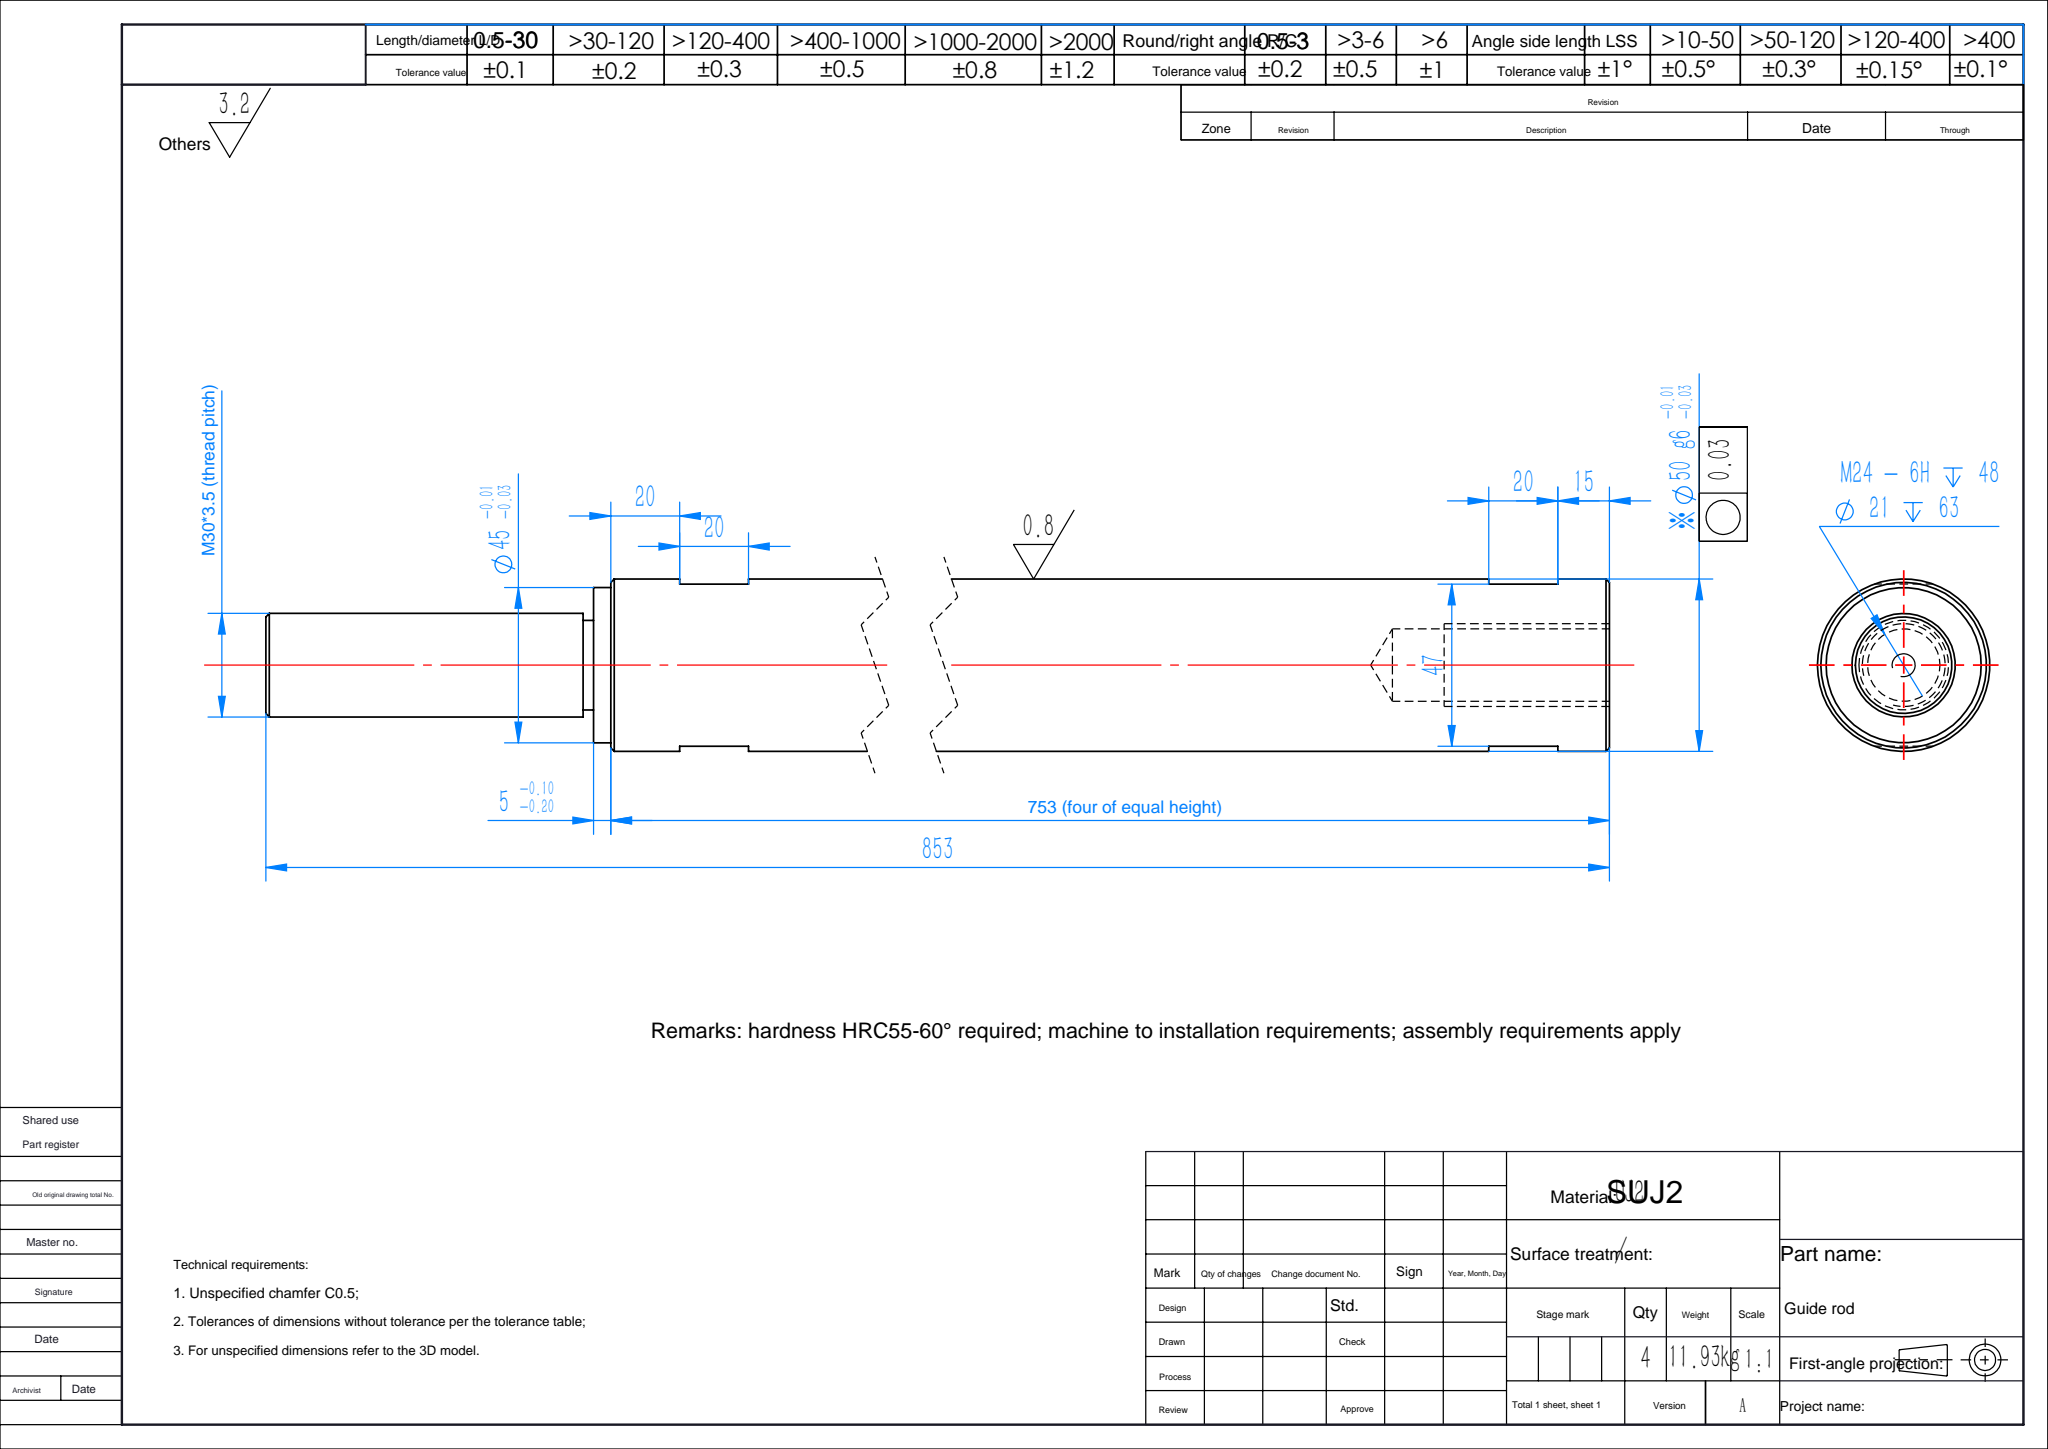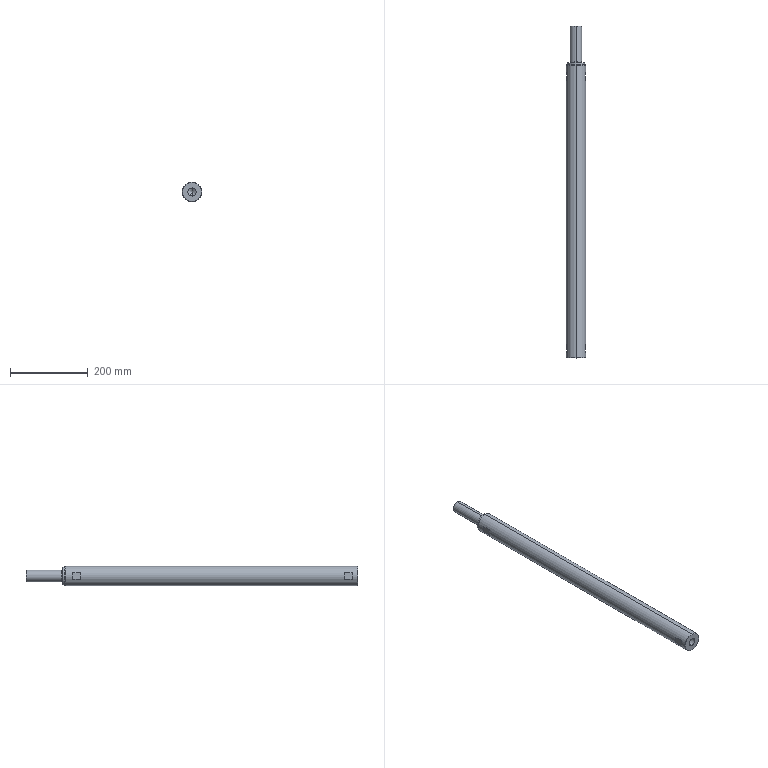Part | SolidWorks | features ICE 5, LibraryFeature 3, Chamfer 1, Extrusion 1, HoleWzd 1 | 1 solid | 35 faces | box 50 x 853 x 50 mm | volume 1528965 mm3 | plane 17 | cylinder 10 | cone 8 | commonest cylinder face diameters 21 x2 26 x2 30 x2 45 x2 50 x2
STEP:
#1=CARTESIAN_POINT('',(0.,384.5,13.));
#2=VERTEX_POINT('',#1);
#3=CARTESIAN_POINT('',(0.,384.5,-13.));
#4=VERTEX_POINT('',#3);
#5=CARTESIAN_POINT('',(0.,384.5,0.));
#6=DIRECTION('',(0.,1.,0.));
#7=DIRECTION('',(0.,0.,1.));
#8=AXIS2_PLACEMENT_3D('',#5,#6,#7);
#9=CIRCLE('',#8,13.);
#10=EDGE_CURVE('',#2,#4,#9,.T.);
#11=ORIENTED_EDGE('',*,*,#10,.F.);
#12=CARTESIAN_POINT('',(0.,381.5,13.));
#13=VERTEX_POINT('',#12);
#14=CARTESIAN_POINT('',(0.,384.5,13.));
#15=DIRECTION('',(0.,-1.,0.));
#16=VECTOR('',#15,1000.);
#17=LINE('',#14,#16);
#18=EDGE_CURVE('',#2,#13,#17,.T.);
#19=ORIENTED_EDGE('',*,*,#18,.T.);
#20=CARTESIAN_POINT('',(0.,381.5,-13.));
#21=VERTEX_POINT('',#20);
#22=CARTESIAN_POINT('',(0.,381.5,0.));
#23=DIRECTION('',(0.,1.,0.));
#24=DIRECTION('',(0.,0.,1.));
#25=AXIS2_PLACEMENT_3D('',#22,#23,#24);
#26=CIRCLE('',#25,13.);
#27=EDGE_CURVE('',#13,#21,#26,.T.);
#28=ORIENTED_EDGE('',*,*,#27,.T.);
#29=CARTESIAN_POINT('',(0.,384.5,-13.));
#30=DIRECTION('',(0.,-1.,0.));
#31=VECTOR('',#30,1000.);
#32=LINE('',#29,#31);
#33=EDGE_CURVE('',#4,#21,#32,.T.);
#34=ORIENTED_EDGE('',*,*,#33,.F.);
#35=EDGE_LOOP('',(#11,#19,#28,#34));
#36=FACE_OUTER_BOUND('',#35,.T.);
#37=CARTESIAN_POINT('',(0.,384.5,0.));
#38=DIRECTION('',(0.,-1.,0.));
#39=DIRECTION('',(0.,0.,-1.));
#40=AXIS2_PLACEMENT_3D('',#37,#38,#39);
#41=CYLINDRICAL_SURFACE('',#40,13.);
#42=ADVANCED_FACE('',(#36),#41,.T.);
#43=CARTESIAN_POINT('',(0.,475.5,-15.));
#44=VERTEX_POINT('',#43);
#45=CARTESIAN_POINT('',(0.,475.5,15.));
#46=VERTEX_POINT('',#45);
#47=CARTESIAN_POINT('',(0.,475.5,0.));
#48=DIRECTION('',(0.,-1.,0.));
#49=DIRECTION('',(0.,0.,1.));
#50=AXIS2_PLACEMENT_3D('',#47,#48,#49);
#51=CIRCLE('',#50,15.);
#52=EDGE_CURVE('',#44,#46,#51,.T.);
#53=ORIENTED_EDGE('',*,*,#52,.T.);
#54=CARTESIAN_POINT('',(0.,384.5,15.));
#55=VERTEX_POINT('',#54);
#56=CARTESIAN_POINT('',(0.,476.5,15.));
#57=DIRECTION('',(0.,-1.,0.));
#58=VECTOR('',#57,1000.);
#59=LINE('',#56,#58);
#60=EDGE_CURVE('',#46,#55,#59,.T.);
#61=ORIENTED_EDGE('',*,*,#60,.T.);
#62=CARTESIAN_POINT('',(0.,384.5,-15.));
#63=VERTEX_POINT('',#62);
#64=CARTESIAN_POINT('',(0.,384.5,0.));
#65=DIRECTION('',(0.,1.,0.));
#66=DIRECTION('',(0.,0.,1.));
#67=AXIS2_PLACEMENT_3D('',#64,#65,#66);
#68=CIRCLE('',#67,15.);
#69=EDGE_CURVE('',#55,#63,#68,.T.);
#70=ORIENTED_EDGE('',*,*,#69,.T.);
#71=CARTESIAN_POINT('',(0.,476.5,-15.));
#72=DIRECTION('',(0.,-1.,0.));
#73=VECTOR('',#72,1000.);
#74=LINE('',#71,#73);
#75=EDGE_CURVE('',#44,#63,#74,.T.);
#76=ORIENTED_EDGE('',*,*,#75,.F.);
#77=EDGE_LOOP('',(#53,#61,#70,#76));
#78=FACE_OUTER_BOUND('',#77,.T.);
#79=CARTESIAN_POINT('',(0.,476.5,0.));
#80=DIRECTION('',(0.,-1.,0.));
#81=DIRECTION('',(0.,0.,-1.));
#82=AXIS2_PLACEMENT_3D('',#79,#80,#81);
#83=CYLINDRICAL_SURFACE('',#82,15.);
#84=ADVANCED_FACE('',(#78),#83,.T.);
#85=CARTESIAN_POINT('',(0.,476.5,14.));
#86=VERTEX_POINT('',#85);
#87=CARTESIAN_POINT('',(0.,476.5,-14.));
#88=VERTEX_POINT('',#87);
#89=CARTESIAN_POINT('',(0.,476.5,0.));
#90=DIRECTION('',(0.,1.,0.));
#91=DIRECTION('',(0.,0.,1.));
#92=AXIS2_PLACEMENT_3D('',#89,#90,#91);
#93=CIRCLE('',#92,14.);
#94=EDGE_CURVE('',#86,#88,#93,.T.);
#95=ORIENTED_EDGE('',*,*,#94,.F.);
#96=CARTESIAN_POINT('',(0.,476.5,14.));
#97=DIRECTION('',(0.,-0.7071,0.7071));
#98=VECTOR('',#97,1000.);
#99=LINE('',#96,#98);
#100=EDGE_CURVE('',#86,#46,#99,.T.);
#101=ORIENTED_EDGE('',*,*,#100,.T.);
#102=ORIENTED_EDGE('',*,*,#52,.F.);
#103=CARTESIAN_POINT('',(0.,476.5,-14.));
#104=DIRECTION('',(0.,-0.7071,-0.7071));
#105=VECTOR('',#104,1000.);
#106=LINE('',#103,#105);
#107=EDGE_CURVE('',#88,#44,#106,.T.);
#108=ORIENTED_EDGE('',*,*,#107,.F.);
#109=EDGE_LOOP('',(#95,#101,#102,#108));
#110=FACE_OUTER_BOUND('',#109,.T.);
#111=CARTESIAN_POINT('',(0.,476.5,0.));
#112=DIRECTION('',(0.,-1.,0.));
#113=DIRECTION('',(0.,0.,-1.));
#114=AXIS2_PLACEMENT_3D('',#111,#112,#113);
#115=CONICAL_SURFACE('',#114,14.,0.7854);
#116=ADVANCED_FACE('',(#110),#115,.T.);
#117=CARTESIAN_POINT('',(0.,381.5,22.5));
#118=VERTEX_POINT('',#117);
#119=CARTESIAN_POINT('',(0.,381.5,-22.5));
#120=VERTEX_POINT('',#119);
#121=CARTESIAN_POINT('',(0.,381.5,0.));
#122=DIRECTION('',(0.,1.,0.));
#123=DIRECTION('',(0.,0.,1.));
#124=AXIS2_PLACEMENT_3D('',#121,#122,#123);
#125=CIRCLE('',#124,22.5);
#126=EDGE_CURVE('',#118,#120,#125,.T.);
#127=ORIENTED_EDGE('',*,*,#126,.F.);
#128=CARTESIAN_POINT('',(0.,376.5,22.5));
#129=VERTEX_POINT('',#128);
#130=CARTESIAN_POINT('',(0.,381.5,22.5));
#131=DIRECTION('',(0.,-1.,0.));
#132=VECTOR('',#131,1000.);
#133=LINE('',#130,#132);
#134=EDGE_CURVE('',#118,#129,#133,.T.);
#135=ORIENTED_EDGE('',*,*,#134,.T.);
#136=CARTESIAN_POINT('',(0.,376.5,-22.5));
#137=VERTEX_POINT('',#136);
#138=CARTESIAN_POINT('',(0.,376.5,0.));
#139=DIRECTION('',(0.,1.,0.));
#140=DIRECTION('',(0.,0.,1.));
#141=AXIS2_PLACEMENT_3D('',#138,#139,#140);
#142=CIRCLE('',#141,22.5);
#143=EDGE_CURVE('',#129,#137,#142,.T.);
#144=ORIENTED_EDGE('',*,*,#143,.T.);
#145=CARTESIAN_POINT('',(0.,381.5,-22.5));
#146=DIRECTION('',(0.,-1.,0.));
#147=VECTOR('',#146,1000.);
#148=LINE('',#145,#147);
#149=EDGE_CURVE('',#120,#137,#148,.T.);
#150=ORIENTED_EDGE('',*,*,#149,.F.);
#151=EDGE_LOOP('',(#127,#135,#144,#150));
#152=FACE_OUTER_BOUND('',#151,.T.);
#153=CARTESIAN_POINT('',(0.,381.5,0.));
#154=DIRECTION('',(0.,-1.,0.));
#155=DIRECTION('',(0.,0.,-1.));
#156=AXIS2_PLACEMENT_3D('',#153,#154,#155);
#157=CYLINDRICAL_SURFACE('',#156,22.5);
#158=ADVANCED_FACE('',(#152),#157,.T.);
#159=CARTESIAN_POINT('',(0.,-376.5,-24.));
#160=VERTEX_POINT('',#159);
#161=CARTESIAN_POINT('',(0.,-376.5,24.));
#162=VERTEX_POINT('',#161);
#163=CARTESIAN_POINT('',(0.,-376.5,0.));
#164=DIRECTION('',(0.,-1.,0.));
#165=DIRECTION('',(0.,0.,1.));
#166=AXIS2_PLACEMENT_3D('',#163,#164,#165);
#167=CIRCLE('',#166,24.);
#168=EDGE_CURVE('',#160,#162,#167,.T.);
#169=ORIENTED_EDGE('',*,*,#168,.F.);
#170=CARTESIAN_POINT('',(0.,-375.5,-25.));
#171=VERTEX_POINT('',#170);
#172=CARTESIAN_POINT('',(0.,-375.5,-25.));
#173=DIRECTION('',(0.,0.7071,-0.7071));
#174=VECTOR('',#173,1000.);
#175=LINE('',#172,#174);
#176=EDGE_CURVE('',#160,#171,#175,.T.);
#177=ORIENTED_EDGE('',*,*,#176,.T.);
#178=CARTESIAN_POINT('',(0.,-375.5,25.));
#179=VERTEX_POINT('',#178);
#180=CARTESIAN_POINT('',(0.,-375.5,0.));
#181=DIRECTION('',(0.,1.,0.));
#182=DIRECTION('',(0.,0.,1.));
#183=AXIS2_PLACEMENT_3D('',#180,#181,#182);
#184=CIRCLE('',#183,25.);
#185=EDGE_CURVE('',#179,#171,#184,.T.);
#186=ORIENTED_EDGE('',*,*,#185,.F.);
#187=CARTESIAN_POINT('',(0.,-375.5,25.));
#188=DIRECTION('',(0.,0.7071,0.7071));
#189=VECTOR('',#188,1000.);
#190=LINE('',#187,#189);
#191=EDGE_CURVE('',#162,#179,#190,.T.);
#192=ORIENTED_EDGE('',*,*,#191,.F.);
#193=EDGE_LOOP('',(#169,#177,#186,#192));
#194=FACE_OUTER_BOUND('',#193,.T.);
#195=CARTESIAN_POINT('',(0.,-375.5,0.));
#196=DIRECTION('',(0.,1.,0.));
#197=DIRECTION('',(0.,0.,1.));
#198=AXIS2_PLACEMENT_3D('',#195,#196,#197);
#199=CONICAL_SURFACE('',#198,25.,0.7854);
#200=ADVANCED_FACE('',(#194),#199,.T.);
#201=CARTESIAN_POINT('',(0.,376.5,24.));
#202=VERTEX_POINT('',#201);
#203=CARTESIAN_POINT('',(0.,376.5,-24.));
#204=VERTEX_POINT('',#203);
#205=CARTESIAN_POINT('',(0.,376.5,0.));
#206=DIRECTION('',(0.,1.,0.));
#207=DIRECTION('',(0.,0.,1.));
#208=AXIS2_PLACEMENT_3D('',#205,#206,#207);
#209=CIRCLE('',#208,24.);
#210=EDGE_CURVE('',#202,#204,#209,.T.);
#211=ORIENTED_EDGE('',*,*,#210,.F.);
#212=CARTESIAN_POINT('',(0.,375.5,25.));
#213=VERTEX_POINT('',#212);
#214=CARTESIAN_POINT('',(0.,376.5,24.));
#215=DIRECTION('',(0.,-0.7071,0.7071));
#216=VECTOR('',#215,1000.);
#217=LINE('',#214,#216);
#218=EDGE_CURVE('',#202,#213,#217,.T.);
#219=ORIENTED_EDGE('',*,*,#218,.T.);
#220=CARTESIAN_POINT('',(0.,375.5,-25.));
#221=VERTEX_POINT('',#220);
#222=CARTESIAN_POINT('',(0.,375.5,0.));
#223=DIRECTION('',(0.,-1.,0.));
#224=DIRECTION('',(0.,0.,1.));
#225=AXIS2_PLACEMENT_3D('',#222,#223,#224);
#226=CIRCLE('',#225,25.);
#227=EDGE_CURVE('',#221,#213,#226,.T.);
#228=ORIENTED_EDGE('',*,*,#227,.F.);
#229=CARTESIAN_POINT('',(0.,376.5,-24.));
#230=DIRECTION('',(0.,-0.7071,-0.7071));
#231=VECTOR('',#230,1000.);
#232=LINE('',#229,#231);
#233=EDGE_CURVE('',#204,#221,#232,.T.);
#234=ORIENTED_EDGE('',*,*,#233,.F.);
#235=EDGE_LOOP('',(#211,#219,#228,#234));
#236=FACE_OUTER_BOUND('',#235,.T.);
#237=CARTESIAN_POINT('',(0.,376.5,0.));
#238=DIRECTION('',(0.,-1.,0.));
#239=DIRECTION('',(0.,0.,-1.));
#240=AXIS2_PLACEMENT_3D('',#237,#238,#239);
#241=CONICAL_SURFACE('',#240,24.,0.7854);
#242=ADVANCED_FACE('',(#236),#241,.T.);
#243=CARTESIAN_POINT('',(0.,-313.5,10.5));
#244=VERTEX_POINT('',#243);
#245=CARTESIAN_POINT('',(0.,-313.5,-10.5));
#246=VERTEX_POINT('',#245);
#247=CARTESIAN_POINT('',(0.,-313.5,0.));
#248=DIRECTION('',(0.,-1.,0.));
#249=DIRECTION('',(0.,0.,-1.));
#250=AXIS2_PLACEMENT_3D('',#247,#248,#249);
#251=CIRCLE('',#250,10.5);
#252=EDGE_CURVE('',#244,#246,#251,.T.);
#253=ORIENTED_EDGE('',*,*,#252,.F.);
#254=CARTESIAN_POINT('',(0.,-376.5,10.5));
#255=VERTEX_POINT('',#254);
#256=CARTESIAN_POINT('',(0.,-376.5,10.5));
#257=DIRECTION('',(0.,-1.,0.));
#258=VECTOR('',#257,1000.);
#259=LINE('',#256,#258);
#260=EDGE_CURVE('',#244,#255,#259,.T.);
#261=ORIENTED_EDGE('',*,*,#260,.T.);
#262=CARTESIAN_POINT('',(0.,-376.5,-10.5));
#263=VERTEX_POINT('',#262);
#264=CARTESIAN_POINT('',(0.,-376.5,0.));
#265=DIRECTION('',(0.,-1.,0.));
#266=DIRECTION('',(0.,0.,-1.));
#267=AXIS2_PLACEMENT_3D('',#264,#265,#266);
#268=CIRCLE('',#267,10.5);
#269=EDGE_CURVE('',#255,#263,#268,.T.);
#270=ORIENTED_EDGE('',*,*,#269,.T.);
#271=CARTESIAN_POINT('',(0.,-376.5,-10.5));
#272=DIRECTION('',(0.,-1.,0.));
#273=VECTOR('',#272,1000.);
#274=LINE('',#271,#273);
#275=EDGE_CURVE('',#246,#263,#274,.T.);
#276=ORIENTED_EDGE('',*,*,#275,.F.);
#277=EDGE_LOOP('',(#253,#261,#270,#276));
#278=FACE_OUTER_BOUND('',#277,.T.);
#279=CARTESIAN_POINT('',(0.,-376.5,0.));
#280=DIRECTION('',(0.,-1.,0.));
#281=DIRECTION('',(0.,0.,-1.));
#282=AXIS2_PLACEMENT_3D('',#279,#280,#281);
#283=CYLINDRICAL_SURFACE('',#282,10.5);
#284=ADVANCED_FACE('',(#278),#283,.F.);
#285=CARTESIAN_POINT('',(0.,-307.191,0.));
#286=VERTEX_POINT('',#285);
#287=CARTESIAN_POINT('',(0.,-313.5,-10.5));
#288=DIRECTION('',(0.,-0.515,-0.8572));
#289=VECTOR('',#288,1000.);
#290=LINE('',#287,#289);
#291=EDGE_CURVE('',#286,#246,#290,.T.);
#292=ORIENTED_EDGE('',*,*,#291,.F.);
#293=CARTESIAN_POINT('',(0.,-313.5,10.5));
#294=DIRECTION('',(0.,-0.515,0.8572));
#295=VECTOR('',#294,1000.);
#296=LINE('',#293,#295);
#297=EDGE_CURVE('',#286,#244,#296,.T.);
#298=ORIENTED_EDGE('',*,*,#297,.T.);
#299=ORIENTED_EDGE('',*,*,#252,.T.);
#300=EDGE_LOOP('',(#292,#298,#299));
#301=FACE_OUTER_BOUND('',#300,.T.);
#302=CARTESIAN_POINT('',(0.,-313.5,0.));
#303=DIRECTION('',(0.,-1.,0.));
#304=DIRECTION('',(0.,0.,-1.));
#305=AXIS2_PLACEMENT_3D('',#302,#303,#304);
#306=CONICAL_SURFACE('',#305,10.5,1.03);
#307=ADVANCED_FACE('',(#301),#306,.F.);
#308=CARTESIAN_POINT('',(23.5,336.5,8.529));
#309=VERTEX_POINT('',#308);
#310=CARTESIAN_POINT('',(23.5,336.5,-8.529));
#311=VERTEX_POINT('',#310);
#312=CARTESIAN_POINT('',(0.,336.5,0.));
#313=DIRECTION('',(0.,1.,0.));
#314=DIRECTION('',(0.,0.,1.));
#315=AXIS2_PLACEMENT_3D('',#312,#313,#314);
#316=CIRCLE('',#315,25.);
#317=EDGE_CURVE('',#309,#311,#316,.T.);
#318=ORIENTED_EDGE('',*,*,#317,.F.);
#319=CARTESIAN_POINT('',(23.5,356.5,8.529));
#320=VERTEX_POINT('',#319);
#321=CARTESIAN_POINT('',(23.5,376.5,8.529));
#322=DIRECTION('',(0.,1.,0.));
#323=VECTOR('',#322,1000.);
#324=LINE('',#321,#323);
#325=EDGE_CURVE('',#309,#320,#324,.T.);
#326=ORIENTED_EDGE('',*,*,#325,.T.);
#327=CARTESIAN_POINT('',(23.5,356.5,-8.529));
#328=VERTEX_POINT('',#327);
#329=CARTESIAN_POINT('',(0.,356.5,0.));
#330=DIRECTION('',(0.,1.,0.));
#331=DIRECTION('',(0.,0.,1.));
#332=AXIS2_PLACEMENT_3D('',#329,#330,#331);
#333=CIRCLE('',#332,25.);
#334=EDGE_CURVE('',#320,#328,#333,.T.);
#335=ORIENTED_EDGE('',*,*,#334,.T.);
#336=CARTESIAN_POINT('',(23.5,376.5,-8.529));
#337=DIRECTION('',(0.,-1.,0.));
#338=VECTOR('',#337,1000.);
#339=LINE('',#336,#338);
#340=EDGE_CURVE('',#328,#311,#339,.T.);
#341=ORIENTED_EDGE('',*,*,#340,.T.);
#342=EDGE_LOOP('',(#318,#326,#335,#341));
#343=FACE_BOUND('',#342,.T.);
#344=CARTESIAN_POINT('',(23.5,-361.5,8.529));
#345=VERTEX_POINT('',#344);
#346=CARTESIAN_POINT('',(23.5,-341.5,8.529));
#347=VERTEX_POINT('',#346);
#348=CARTESIAN_POINT('',(23.5,376.5,8.529));
#349=DIRECTION('',(0.,1.,0.));
#350=VECTOR('',#349,1000.);
#351=LINE('',#348,#350);
#352=EDGE_CURVE('',#345,#347,#351,.T.);
#353=ORIENTED_EDGE('',*,*,#352,.T.);
#354=CARTESIAN_POINT('',(23.5,-341.5,-8.529));
#355=VERTEX_POINT('',#354);
#356=CARTESIAN_POINT('',(0.,-341.5,0.));
#357=DIRECTION('',(0.,1.,0.));
#358=DIRECTION('',(0.,0.,1.));
#359=AXIS2_PLACEMENT_3D('',#356,#357,#358);
#360=CIRCLE('',#359,25.);
#361=EDGE_CURVE('',#347,#355,#360,.T.);
#362=ORIENTED_EDGE('',*,*,#361,.T.);
#363=CARTESIAN_POINT('',(23.5,-361.5,-8.529));
#364=VERTEX_POINT('',#363);
#365=CARTESIAN_POINT('',(23.5,376.5,-8.529));
#366=DIRECTION('',(0.,-1.,0.));
#367=VECTOR('',#366,1000.);
#368=LINE('',#365,#367);
#369=EDGE_CURVE('',#355,#364,#368,.T.);
#370=ORIENTED_EDGE('',*,*,#369,.T.);
#371=CARTESIAN_POINT('',(0.,-361.5,0.));
#372=DIRECTION('',(0.,1.,0.));
#373=DIRECTION('',(0.,0.,1.));
#374=AXIS2_PLACEMENT_3D('',#371,#372,#373);
#375=CIRCLE('',#374,25.);
#376=EDGE_CURVE('',#345,#364,#375,.T.);
#377=ORIENTED_EDGE('',*,*,#376,.F.);
#378=EDGE_LOOP('',(#353,#362,#370,#377));
#379=FACE_BOUND('',#378,.T.);
#380=ORIENTED_EDGE('',*,*,#227,.T.);
#381=CARTESIAN_POINT('',(0.,376.5,25.));
#382=DIRECTION('',(0.,-1.,0.));
#383=VECTOR('',#382,1000.);
#384=LINE('',#381,#383);
#385=EDGE_CURVE('',#213,#179,#384,.T.);
#386=ORIENTED_EDGE('',*,*,#385,.T.);
#387=ORIENTED_EDGE('',*,*,#185,.T.);
#388=CARTESIAN_POINT('',(0.,376.5,-25.));
#389=DIRECTION('',(0.,-1.,0.));
#390=VECTOR('',#389,1000.);
#391=LINE('',#388,#390);
#392=EDGE_CURVE('',#221,#171,#391,.T.);
#393=ORIENTED_EDGE('',*,*,#392,.F.);
#394=EDGE_LOOP('',(#380,#386,#387,#393));
#395=FACE_OUTER_BOUND('',#394,.T.);
#396=CARTESIAN_POINT('',(0.,376.5,0.));
#397=DIRECTION('',(0.,-1.,0.));
#398=DIRECTION('',(0.,0.,-1.));
#399=AXIS2_PLACEMENT_3D('',#396,#397,#398);
#400=CYLINDRICAL_SURFACE('',#399,25.);
#401=ADVANCED_FACE('',(#343,#379,#395),#400,.T.);
#402=ORIENTED_EDGE('',*,*,#385,.F.);
#403=CARTESIAN_POINT('',(0.,375.5,0.));
#404=DIRECTION('',(0.,-1.,0.));
#405=DIRECTION('',(0.,0.,1.));
#406=AXIS2_PLACEMENT_3D('',#403,#404,#405);
#407=CIRCLE('',#406,25.);
#408=EDGE_CURVE('',#213,#221,#407,.T.);
#409=ORIENTED_EDGE('',*,*,#408,.T.);
#410=ORIENTED_EDGE('',*,*,#392,.T.);
#411=CARTESIAN_POINT('',(0.,-375.5,0.));
#412=DIRECTION('',(0.,1.,0.));
#413=DIRECTION('',(0.,0.,1.));
#414=AXIS2_PLACEMENT_3D('',#411,#412,#413);
#415=CIRCLE('',#414,25.);
#416=EDGE_CURVE('',#171,#179,#415,.T.);
#417=ORIENTED_EDGE('',*,*,#416,.T.);
#418=EDGE_LOOP('',(#402,#409,#410,#417));
#419=FACE_OUTER_BOUND('',#418,.T.);
#420=CARTESIAN_POINT('',(-23.5,356.5,8.529));
#421=VERTEX_POINT('',#420);
#422=CARTESIAN_POINT('',(-23.5,336.5,8.529));
#423=VERTEX_POINT('',#422);
#424=CARTESIAN_POINT('',(-23.5,376.5,8.529));
#425=DIRECTION('',(0.,-1.,0.));
#426=VECTOR('',#425,1000.);
#427=LINE('',#424,#426);
#428=EDGE_CURVE('',#421,#423,#427,.T.);
#429=ORIENTED_EDGE('',*,*,#428,.T.);
#430=CARTESIAN_POINT('',(-23.5,336.5,-8.529));
#431=VERTEX_POINT('',#430);
#432=CARTESIAN_POINT('',(0.,336.5,0.));
#433=DIRECTION('',(0.,-1.,0.));
#434=DIRECTION('',(0.,0.,-1.));
#435=AXIS2_PLACEMENT_3D('',#432,#433,#434);
#436=CIRCLE('',#435,25.);
#437=EDGE_CURVE('',#423,#431,#436,.T.);
#438=ORIENTED_EDGE('',*,*,#437,.T.);
#439=CARTESIAN_POINT('',(-23.5,356.5,-8.529));
#440=VERTEX_POINT('',#439);
#441=CARTESIAN_POINT('',(-23.5,376.5,-8.529));
#442=DIRECTION('',(0.,1.,0.));
#443=VECTOR('',#442,1000.);
#444=LINE('',#441,#443);
#445=EDGE_CURVE('',#431,#440,#444,.T.);
#446=ORIENTED_EDGE('',*,*,#445,.T.);
#447=CARTESIAN_POINT('',(0.,356.5,0.));
#448=DIRECTION('',(0.,-1.,0.));
#449=DIRECTION('',(0.,0.,-1.));
#450=AXIS2_PLACEMENT_3D('',#447,#448,#449);
#451=CIRCLE('',#450,25.);
#452=EDGE_CURVE('',#421,#440,#451,.T.);
#453=ORIENTED_EDGE('',*,*,#452,.F.);
#454=EDGE_LOOP('',(#429,#438,#446,#453));
#455=FACE_BOUND('',#454,.T.);
#456=CARTESIAN_POINT('',(-23.5,-341.5,8.529));
#457=VERTEX_POINT('',#456);
#458=CARTESIAN_POINT('',(-23.5,-341.5,-8.529));
#459=VERTEX_POINT('',#458);
#460=CARTESIAN_POINT('',(0.,-341.5,0.));
#461=DIRECTION('',(0.,-1.,0.));
#462=DIRECTION('',(0.,0.,-1.));
#463=AXIS2_PLACEMENT_3D('',#460,#461,#462);
#464=CIRCLE('',#463,25.);
#465=EDGE_CURVE('',#457,#459,#464,.T.);
#466=ORIENTED_EDGE('',*,*,#465,.F.);
#467=CARTESIAN_POINT('',(-23.5,-361.5,8.529));
#468=VERTEX_POINT('',#467);
#469=CARTESIAN_POINT('',(-23.5,376.5,8.529));
#470=DIRECTION('',(0.,-1.,0.));
#471=VECTOR('',#470,1000.);
#472=LINE('',#469,#471);
#473=EDGE_CURVE('',#457,#468,#472,.T.);
#474=ORIENTED_EDGE('',*,*,#473,.T.);
#475=CARTESIAN_POINT('',(-23.5,-361.5,-8.529));
#476=VERTEX_POINT('',#475);
#477=CARTESIAN_POINT('',(0.,-361.5,0.));
#478=DIRECTION('',(0.,-1.,0.));
#479=DIRECTION('',(0.,0.,-1.));
#480=AXIS2_PLACEMENT_3D('',#477,#478,#479);
#481=CIRCLE('',#480,25.);
#482=EDGE_CURVE('',#468,#476,#481,.T.);
#483=ORIENTED_EDGE('',*,*,#482,.T.);
#484=CARTESIAN_POINT('',(-23.5,376.5,-8.529));
#485=DIRECTION('',(0.,1.,0.));
#486=VECTOR('',#485,1000.);
#487=LINE('',#484,#486);
#488=EDGE_CURVE('',#476,#459,#487,.T.);
#489=ORIENTED_EDGE('',*,*,#488,.T.);
#490=EDGE_LOOP('',(#466,#474,#483,#489));
#491=FACE_BOUND('',#490,.T.);
#492=CARTESIAN_POINT('',(0.,376.5,0.));
#493=DIRECTION('',(0.,-1.,0.));
#494=DIRECTION('',(0.,0.,-1.));
#495=AXIS2_PLACEMENT_3D('',#492,#493,#494);
#496=CYLINDRICAL_SURFACE('',#495,25.);
#497=ADVANCED_FACE('',(#419,#455,#491),#496,.T.);
#498=CARTESIAN_POINT('',(0.,376.5,0.));
#499=DIRECTION('',(0.,1.,0.));
#500=DIRECTION('',(0.,0.,1.));
#501=AXIS2_PLACEMENT_3D('',#498,#499,#500);
#502=CIRCLE('',#501,22.5);
#503=EDGE_CURVE('',#137,#129,#502,.T.);
#504=ORIENTED_EDGE('',*,*,#503,.F.);
#505=ORIENTED_EDGE('',*,*,#143,.F.);
#506=EDGE_LOOP('',(#504,#505));
#507=FACE_BOUND('',#506,.T.);
#508=CARTESIAN_POINT('',(0.,376.5,0.));
#509=DIRECTION('',(0.,1.,0.));
#510=DIRECTION('',(0.,0.,1.));
#511=AXIS2_PLACEMENT_3D('',#508,#509,#510);
#512=CIRCLE('',#511,24.);
#513=EDGE_CURVE('',#204,#202,#512,.T.);
#514=ORIENTED_EDGE('',*,*,#513,.T.);
#515=ORIENTED_EDGE('',*,*,#210,.T.);
#516=EDGE_LOOP('',(#514,#515));
#517=FACE_OUTER_BOUND('',#516,.T.);
#518=CARTESIAN_POINT('',(0.,376.5,0.));
#519=DIRECTION('',(0.,1.,0.));
#520=DIRECTION('',(0.,0.,1.));
#521=AXIS2_PLACEMENT_3D('',#518,#519,#520);
#522=PLANE('',#521);
#523=ADVANCED_FACE('',(#507,#517),#522,.T.);
#524=CARTESIAN_POINT('',(0.,-376.5,0.));
#525=DIRECTION('',(0.,-1.,0.));
#526=DIRECTION('',(0.,0.,1.));
#527=AXIS2_PLACEMENT_3D('',#524,#525,#526);
#528=CIRCLE('',#527,24.);
#529=EDGE_CURVE('',#162,#160,#528,.T.);
#530=ORIENTED_EDGE('',*,*,#529,.T.);
#531=ORIENTED_EDGE('',*,*,#168,.T.);
#532=EDGE_LOOP('',(#530,#531));
#533=FACE_OUTER_BOUND('',#532,.T.);
#534=CARTESIAN_POINT('',(0.,-376.5,0.));
#535=DIRECTION('',(0.,-1.,0.));
#536=DIRECTION('',(0.,0.,-1.));
#537=AXIS2_PLACEMENT_3D('',#534,#535,#536);
#538=CIRCLE('',#537,10.5);
#539=EDGE_CURVE('',#263,#255,#538,.T.);
#540=ORIENTED_EDGE('',*,*,#539,.F.);
#541=ORIENTED_EDGE('',*,*,#269,.F.);
#542=EDGE_LOOP('',(#540,#541));
#543=FACE_BOUND('',#542,.T.);
#544=CARTESIAN_POINT('',(0.,-376.5,0.));
#545=DIRECTION('',(0.,1.,0.));
#546=DIRECTION('',(0.,0.,1.));
#547=AXIS2_PLACEMENT_3D('',#544,#545,#546);
#548=PLANE('',#547);
#549=ADVANCED_FACE('',(#533,#543),#548,.F.);
#550=ORIENTED_EDGE('',*,*,#297,.F.);
#551=ORIENTED_EDGE('',*,*,#291,.T.);
#552=CARTESIAN_POINT('',(0.,-313.5,0.));
#553=DIRECTION('',(0.,-1.,0.));
#554=DIRECTION('',(0.,0.,-1.));
#555=AXIS2_PLACEMENT_3D('',#552,#553,#554);
#556=CIRCLE('',#555,10.5);
#557=EDGE_CURVE('',#246,#244,#556,.T.);
#558=ORIENTED_EDGE('',*,*,#557,.T.);
#559=EDGE_LOOP('',(#550,#551,#558));
#560=FACE_OUTER_BOUND('',#559,.T.);
#561=CARTESIAN_POINT('',(0.,-313.5,0.));
#562=DIRECTION('',(0.,-1.,0.));
#563=DIRECTION('',(0.,0.,-1.));
#564=AXIS2_PLACEMENT_3D('',#561,#562,#563);
#565=CONICAL_SURFACE('',#564,10.5,1.03);
#566=ADVANCED_FACE('',(#560),#565,.F.);
#567=ORIENTED_EDGE('',*,*,#260,.F.);
#568=ORIENTED_EDGE('',*,*,#557,.F.);
#569=ORIENTED_EDGE('',*,*,#275,.T.);
#570=ORIENTED_EDGE('',*,*,#539,.T.);
#571=EDGE_LOOP('',(#567,#568,#569,#570));
#572=FACE_OUTER_BOUND('',#571,.T.);
#573=CARTESIAN_POINT('',(0.,-376.5,0.));
#574=DIRECTION('',(0.,-1.,0.));
#575=DIRECTION('',(0.,0.,-1.));
#576=AXIS2_PLACEMENT_3D('',#573,#574,#575);
#577=CYLINDRICAL_SURFACE('',#576,10.5);
#578=ADVANCED_FACE('',(#572),#577,.F.);
#579=CARTESIAN_POINT('',(23.5,356.5,-25.));
#580=DIRECTION('',(0.,0.,1.));
#581=VECTOR('',#580,1000.);
#582=LINE('',#579,#581);
#583=EDGE_CURVE('',#328,#320,#582,.T.);
#584=ORIENTED_EDGE('',*,*,#583,.T.);
#585=ORIENTED_EDGE('',*,*,#325,.F.);
#586=CARTESIAN_POINT('',(23.5,336.5,-25.));
#587=DIRECTION('',(0.,0.,1.));
#588=VECTOR('',#587,1000.);
#589=LINE('',#586,#588);
#590=EDGE_CURVE('',#311,#309,#589,.T.);
#591=ORIENTED_EDGE('',*,*,#590,.F.);
#592=ORIENTED_EDGE('',*,*,#340,.F.);
#593=EDGE_LOOP('',(#584,#585,#591,#592));
#594=FACE_OUTER_BOUND('',#593,.T.);
#595=CARTESIAN_POINT('',(23.5,336.5,-25.));
#596=DIRECTION('',(-1.,0.,0.));
#597=DIRECTION('',(0.,0.,1.));
#598=AXIS2_PLACEMENT_3D('',#595,#596,#597);
#599=PLANE('',#598);
#600=ADVANCED_FACE('',(#594),#599,.F.);
#601=ORIENTED_EDGE('',*,*,#590,.T.);
#602=ORIENTED_EDGE('',*,*,#317,.T.);
#603=EDGE_LOOP('',(#601,#602));
#604=FACE_OUTER_BOUND('',#603,.T.);
#605=CARTESIAN_POINT('',(0.,336.5,0.));
#606=DIRECTION('',(0.,1.,0.));
#607=DIRECTION('',(0.,0.,1.));
#608=AXIS2_PLACEMENT_3D('',#605,#606,#607);
#609=PLANE('',#608);
#610=ADVANCED_FACE('',(#604),#609,.T.);
#611=ORIENTED_EDGE('',*,*,#583,.F.);
#612=ORIENTED_EDGE('',*,*,#334,.F.);
#613=EDGE_LOOP('',(#611,#612));
#614=FACE_OUTER_BOUND('',#613,.T.);
#615=CARTESIAN_POINT('',(0.,356.5,0.));
#616=DIRECTION('',(0.,1.,0.));
#617=DIRECTION('',(0.,0.,1.));
#618=AXIS2_PLACEMENT_3D('',#615,#616,#617);
#619=PLANE('',#618);
#620=ADVANCED_FACE('',(#614),#619,.F.);
#621=CARTESIAN_POINT('',(-23.5,356.5,-25.));
#622=DIRECTION('',(0.,0.,-1.));
#623=VECTOR('',#622,1000.);
#624=LINE('',#621,#623);
#625=EDGE_CURVE('',#421,#440,#624,.T.);
#626=ORIENTED_EDGE('',*,*,#625,.T.);
#627=ORIENTED_EDGE('',*,*,#445,.F.);
#628=CARTESIAN_POINT('',(-23.5,336.5,-25.));
#629=DIRECTION('',(0.,0.,-1.));
#630=VECTOR('',#629,1000.);
#631=LINE('',#628,#630);
#632=EDGE_CURVE('',#423,#431,#631,.T.);
#633=ORIENTED_EDGE('',*,*,#632,.F.);
#634=ORIENTED_EDGE('',*,*,#428,.F.);
#635=EDGE_LOOP('',(#626,#627,#633,#634));
#636=FACE_OUTER_BOUND('',#635,.T.);
#637=CARTESIAN_POINT('',(-23.5,336.5,-25.));
#638=DIRECTION('',(1.,0.,0.));
#639=DIRECTION('',(0.,0.,-1.));
#640=AXIS2_PLACEMENT_3D('',#637,#638,#639);
#641=PLANE('',#640);
#642=ADVANCED_FACE('',(#636),#641,.F.);
#643=ORIENTED_EDGE('',*,*,#632,.T.);
#644=ORIENTED_EDGE('',*,*,#437,.F.);
#645=EDGE_LOOP('',(#643,#644));
#646=FACE_OUTER_BOUND('',#645,.T.);
#647=CARTESIAN_POINT('',(0.,336.5,0.));
#648=DIRECTION('',(0.,-1.,0.));
#649=DIRECTION('',(0.,0.,-1.));
#650=AXIS2_PLACEMENT_3D('',#647,#648,#649);
#651=PLANE('',#650);
#652=ADVANCED_FACE('',(#646),#651,.F.);
#653=ORIENTED_EDGE('',*,*,#625,.F.);
#654=ORIENTED_EDGE('',*,*,#452,.T.);
#655=EDGE_LOOP('',(#653,#654));
#656=FACE_OUTER_BOUND('',#655,.T.);
#657=CARTESIAN_POINT('',(0.,356.5,0.));
#658=DIRECTION('',(0.,-1.,0.));
#659=DIRECTION('',(0.,0.,-1.));
#660=AXIS2_PLACEMENT_3D('',#657,#658,#659);
#661=PLANE('',#660);
#662=ADVANCED_FACE('',(#656),#661,.T.);
#663=CARTESIAN_POINT('',(-23.5,-341.5,-25.));
#664=DIRECTION('',(0.,0.,1.));
#665=VECTOR('',#664,1000.);
#666=LINE('',#663,#665);
#667=EDGE_CURVE('',#459,#457,#666,.T.);
#668=ORIENTED_EDGE('',*,*,#667,.F.);
#669=ORIENTED_EDGE('',*,*,#488,.F.);
#670=CARTESIAN_POINT('',(-23.5,-361.5,-25.));
#671=DIRECTION('',(0.,0.,1.));
#672=VECTOR('',#671,1000.);
#673=LINE('',#670,#672);
#674=EDGE_CURVE('',#476,#468,#673,.T.);
#675=ORIENTED_EDGE('',*,*,#674,.T.);
#676=ORIENTED_EDGE('',*,*,#473,.F.);
#677=EDGE_LOOP('',(#668,#669,#675,#676));
#678=FACE_OUTER_BOUND('',#677,.T.);
#679=CARTESIAN_POINT('',(-23.5,-341.5,-25.));
#680=DIRECTION('',(1.,0.,0.));
#681=DIRECTION('',(0.,0.,-1.));
#682=AXIS2_PLACEMENT_3D('',#679,#680,#681);
#683=PLANE('',#682);
#684=ADVANCED_FACE('',(#678),#683,.F.);
#685=ORIENTED_EDGE('',*,*,#667,.T.);
#686=ORIENTED_EDGE('',*,*,#465,.T.);
#687=EDGE_LOOP('',(#685,#686));
#688=FACE_OUTER_BOUND('',#687,.T.);
#689=CARTESIAN_POINT('',(0.,-341.5,0.));
#690=DIRECTION('',(0.,-1.,0.));
#691=DIRECTION('',(0.,0.,-1.));
#692=AXIS2_PLACEMENT_3D('',#689,#690,#691);
#693=PLANE('',#692);
#694=ADVANCED_FACE('',(#688),#693,.T.);
#695=ORIENTED_EDGE('',*,*,#674,.F.);
#696=ORIENTED_EDGE('',*,*,#482,.F.);
#697=EDGE_LOOP('',(#695,#696));
#698=FACE_OUTER_BOUND('',#697,.T.);
#699=CARTESIAN_POINT('',(0.,-361.5,0.));
#700=DIRECTION('',(0.,-1.,0.));
#701=DIRECTION('',(0.,0.,-1.));
#702=AXIS2_PLACEMENT_3D('',#699,#700,#701);
#703=PLANE('',#702);
#704=ADVANCED_FACE('',(#698),#703,.F.);
#705=CARTESIAN_POINT('',(23.5,-341.5,-25.));
#706=DIRECTION('',(0.,0.,-1.));
#707=VECTOR('',#706,1000.);
#708=LINE('',#705,#707);
#709=EDGE_CURVE('',#347,#355,#708,.T.);
#710=ORIENTED_EDGE('',*,*,#709,.F.);
#711=ORIENTED_EDGE('',*,*,#352,.F.);
#712=CARTESIAN_POINT('',(23.5,-361.5,-25.));
#713=DIRECTION('',(0.,0.,-1.));
#714=VECTOR('',#713,1000.);
#715=LINE('',#712,#714);
#716=EDGE_CURVE('',#345,#364,#715,.T.);
#717=ORIENTED_EDGE('',*,*,#716,.T.);
#718=ORIENTED_EDGE('',*,*,#369,.F.);
#719=EDGE_LOOP('',(#710,#711,#717,#718));
#720=FACE_OUTER_BOUND('',#719,.T.);
#721=CARTESIAN_POINT('',(23.5,-341.5,-25.));
#722=DIRECTION('',(-1.,0.,0.));
#723=DIRECTION('',(0.,0.,1.));
#724=AXIS2_PLACEMENT_3D('',#721,#722,#723);
#725=PLANE('',#724);
#726=ADVANCED_FACE('',(#720),#725,.F.);
#727=ORIENTED_EDGE('',*,*,#709,.T.);
#728=ORIENTED_EDGE('',*,*,#361,.F.);
#729=EDGE_LOOP('',(#727,#728));
#730=FACE_OUTER_BOUND('',#729,.T.);
#731=CARTESIAN_POINT('',(0.,-341.5,0.));
#732=DIRECTION('',(0.,1.,0.));
#733=DIRECTION('',(0.,0.,1.));
#734=AXIS2_PLACEMENT_3D('',#731,#732,#733);
#735=PLANE('',#734);
#736=ADVANCED_FACE('',(#730),#735,.F.);
#737=ORIENTED_EDGE('',*,*,#716,.F.);
#738=ORIENTED_EDGE('',*,*,#376,.T.);
#739=EDGE_LOOP('',(#737,#738));
#740=FACE_OUTER_BOUND('',#739,.T.);
#741=CARTESIAN_POINT('',(0.,-361.5,0.));
#742=DIRECTION('',(0.,1.,0.));
#743=DIRECTION('',(0.,0.,1.));
#744=AXIS2_PLACEMENT_3D('',#741,#742,#743);
#745=PLANE('',#744);
#746=ADVANCED_FACE('',(#740),#745,.T.);
#747=ORIENTED_EDGE('',*,*,#218,.F.);
#748=ORIENTED_EDGE('',*,*,#513,.F.);
#749=ORIENTED_EDGE('',*,*,#233,.T.);
#750=ORIENTED_EDGE('',*,*,#408,.F.);
#751=EDGE_LOOP('',(#747,#748,#749,#750));
#752=FACE_OUTER_BOUND('',#751,.T.);
#753=CARTESIAN_POINT('',(0.,376.5,0.));
#754=DIRECTION('',(0.,-1.,0.));
#755=DIRECTION('',(0.,0.,-1.));
#756=AXIS2_PLACEMENT_3D('',#753,#754,#755);
#757=CONICAL_SURFACE('',#756,24.,0.7854);
#758=ADVANCED_FACE('',(#752),#757,.T.);
#759=ORIENTED_EDGE('',*,*,#176,.F.);
#760=ORIENTED_EDGE('',*,*,#529,.F.);
#761=ORIENTED_EDGE('',*,*,#191,.T.);
#762=ORIENTED_EDGE('',*,*,#416,.F.);
#763=EDGE_LOOP('',(#759,#760,#761,#762));
#764=FACE_OUTER_BOUND('',#763,.T.);
#765=CARTESIAN_POINT('',(0.,-375.5,0.));
#766=DIRECTION('',(0.,1.,0.));
#767=DIRECTION('',(0.,0.,1.));
#768=AXIS2_PLACEMENT_3D('',#765,#766,#767);
#769=CONICAL_SURFACE('',#768,25.,0.7854);
#770=ADVANCED_FACE('',(#764),#769,.T.);
#771=ORIENTED_EDGE('',*,*,#134,.F.);
#772=CARTESIAN_POINT('',(0.,381.5,0.));
#773=DIRECTION('',(0.,1.,0.));
#774=DIRECTION('',(0.,0.,1.));
#775=AXIS2_PLACEMENT_3D('',#772,#773,#774);
#776=CIRCLE('',#775,22.5);
#777=EDGE_CURVE('',#120,#118,#776,.T.);
#778=ORIENTED_EDGE('',*,*,#777,.F.);
#779=ORIENTED_EDGE('',*,*,#149,.T.);
#780=ORIENTED_EDGE('',*,*,#503,.T.);
#781=EDGE_LOOP('',(#771,#778,#779,#780));
#782=FACE_OUTER_BOUND('',#781,.T.);
#783=CARTESIAN_POINT('',(0.,381.5,0.));
#784=DIRECTION('',(0.,-1.,0.));
#785=DIRECTION('',(0.,0.,-1.));
#786=AXIS2_PLACEMENT_3D('',#783,#784,#785);
#787=CYLINDRICAL_SURFACE('',#786,22.5);
#788=ADVANCED_FACE('',(#782),#787,.T.);
#789=CARTESIAN_POINT('',(0.,476.5,0.));
#790=DIRECTION('',(0.,1.,0.));
#791=DIRECTION('',(0.,0.,1.));
#792=AXIS2_PLACEMENT_3D('',#789,#790,#791);
#793=CIRCLE('',#792,14.);
#794=EDGE_CURVE('',#88,#86,#793,.T.);
#795=ORIENTED_EDGE('',*,*,#794,.T.);
#796=ORIENTED_EDGE('',*,*,#94,.T.);
#797=EDGE_LOOP('',(#795,#796));
#798=FACE_OUTER_BOUND('',#797,.T.);
#799=CARTESIAN_POINT('',(0.,476.5,0.));
#800=DIRECTION('',(0.,1.,0.));
#801=DIRECTION('',(0.,0.,1.));
#802=AXIS2_PLACEMENT_3D('',#799,#800,#801);
#803=PLANE('',#802);
#804=ADVANCED_FACE('',(#798),#803,.T.);
#805=ORIENTED_EDGE('',*,*,#100,.F.);
#806=ORIENTED_EDGE('',*,*,#794,.F.);
#807=ORIENTED_EDGE('',*,*,#107,.T.);
#808=CARTESIAN_POINT('',(0.,475.5,0.));
#809=DIRECTION('',(0.,-1.,0.));
#810=DIRECTION('',(0.,0.,1.));
#811=AXIS2_PLACEMENT_3D('',#808,#809,#810);
#812=CIRCLE('',#811,15.);
#813=EDGE_CURVE('',#46,#44,#812,.T.);
#814=ORIENTED_EDGE('',*,*,#813,.F.);
#815=EDGE_LOOP('',(#805,#806,#807,#814));
#816=FACE_OUTER_BOUND('',#815,.T.);
#817=CARTESIAN_POINT('',(0.,476.5,0.));
#818=DIRECTION('',(0.,-1.,0.));
#819=DIRECTION('',(0.,0.,-1.));
#820=AXIS2_PLACEMENT_3D('',#817,#818,#819);
#821=CONICAL_SURFACE('',#820,14.,0.7854);
#822=ADVANCED_FACE('',(#816),#821,.T.);
#823=ORIENTED_EDGE('',*,*,#60,.F.);
#824=ORIENTED_EDGE('',*,*,#813,.T.);
#825=ORIENTED_EDGE('',*,*,#75,.T.);
#826=CARTESIAN_POINT('',(0.,384.5,0.));
#827=DIRECTION('',(0.,1.,0.));
#828=DIRECTION('',(0.,0.,1.));
#829=AXIS2_PLACEMENT_3D('',#826,#827,#828);
#830=CIRCLE('',#829,15.);
#831=EDGE_CURVE('',#63,#55,#830,.T.);
#832=ORIENTED_EDGE('',*,*,#831,.T.);
#833=EDGE_LOOP('',(#823,#824,#825,#832));
#834=FACE_OUTER_BOUND('',#833,.T.);
#835=CARTESIAN_POINT('',(0.,476.5,0.));
#836=DIRECTION('',(0.,-1.,0.));
#837=DIRECTION('',(0.,0.,-1.));
#838=AXIS2_PLACEMENT_3D('',#835,#836,#837);
#839=CYLINDRICAL_SURFACE('',#838,15.);
#840=ADVANCED_FACE('',(#834),#839,.T.);
#841=ORIENTED_EDGE('',*,*,#831,.F.);
#842=ORIENTED_EDGE('',*,*,#69,.F.);
#843=EDGE_LOOP('',(#841,#842));
#844=FACE_OUTER_BOUND('',#843,.T.);
#845=CARTESIAN_POINT('',(0.,384.5,0.));
#846=DIRECTION('',(0.,1.,0.));
#847=DIRECTION('',(0.,0.,1.));
#848=AXIS2_PLACEMENT_3D('',#845,#846,#847);
#849=CIRCLE('',#848,13.);
#850=EDGE_CURVE('',#4,#2,#849,.T.);
#851=ORIENTED_EDGE('',*,*,#850,.T.);
#852=ORIENTED_EDGE('',*,*,#10,.T.);
#853=EDGE_LOOP('',(#851,#852));
#854=FACE_BOUND('',#853,.T.);
#855=CARTESIAN_POINT('',(0.,384.5,0.));
#856=DIRECTION('',(0.,1.,0.));
#857=DIRECTION('',(0.,0.,1.));
#858=AXIS2_PLACEMENT_3D('',#855,#856,#857);
#859=PLANE('',#858);
#860=ADVANCED_FACE('',(#844,#854),#859,.F.);
#861=ORIENTED_EDGE('',*,*,#18,.F.);
#862=ORIENTED_EDGE('',*,*,#850,.F.);
#863=ORIENTED_EDGE('',*,*,#33,.T.);
#864=CARTESIAN_POINT('',(0.,381.5,0.));
#865=DIRECTION('',(0.,1.,0.));
#866=DIRECTION('',(0.,0.,1.));
#867=AXIS2_PLACEMENT_3D('',#864,#865,#866);
#868=CIRCLE('',#867,13.);
#869=EDGE_CURVE('',#21,#13,#868,.T.);
#870=ORIENTED_EDGE('',*,*,#869,.T.);
#871=EDGE_LOOP('',(#861,#862,#863,#870));
#872=FACE_OUTER_BOUND('',#871,.T.);
#873=CARTESIAN_POINT('',(0.,384.5,0.));
#874=DIRECTION('',(0.,-1.,0.));
#875=DIRECTION('',(0.,0.,-1.));
#876=AXIS2_PLACEMENT_3D('',#873,#874,#875);
#877=CYLINDRICAL_SURFACE('',#876,13.);
#878=ADVANCED_FACE('',(#872),#877,.T.);
#879=ORIENTED_EDGE('',*,*,#869,.F.);
#880=ORIENTED_EDGE('',*,*,#27,.F.);
#881=EDGE_LOOP('',(#879,#880));
#882=FACE_BOUND('',#881,.T.);
#883=ORIENTED_EDGE('',*,*,#777,.T.);
#884=ORIENTED_EDGE('',*,*,#126,.T.);
#885=EDGE_LOOP('',(#883,#884));
#886=FACE_OUTER_BOUND('',#885,.T.);
#887=CARTESIAN_POINT('',(0.,381.5,0.));
#888=DIRECTION('',(0.,1.,0.));
#889=DIRECTION('',(0.,0.,1.));
#890=AXIS2_PLACEMENT_3D('',#887,#888,#889);
#891=PLANE('',#890);
#892=ADVANCED_FACE('',(#882,#886),#891,.T.);
#893=CLOSED_SHELL('',(#42,#84,#116,#158,#200,#242,#284,#307,#401,#497,#523,#549,#566,#578,#600,#610,#620,#642,#652,#662,#684,#694,#704,#726,#736,#746,#758,#770,#788,#804,#822,#840,#860,#878,#892));
#894=MANIFOLD_SOLID_BREP('',#893);
#895=CARTESIAN_POINT('',(0.,0.,0.));
#896=DIRECTION('',(0.,0.,1.));
#897=DIRECTION('',(1.,0.,0.));
#898=AXIS2_PLACEMENT_3D('',#895,#896,#897);
#899=(LENGTH_UNIT()NAMED_UNIT(*)SI_UNIT(.MILLI.,.METRE.));
#900=UNCERTAINTY_MEASURE_WITH_UNIT(LENGTH_MEASURE(0.00001),#899,'','');
#901=(NAMED_UNIT(*)PLANE_ANGLE_UNIT()SI_UNIT($,.RADIAN.));
#902=(NAMED_UNIT(*)SI_UNIT($,.STERADIAN.)SOLID_ANGLE_UNIT());
#903=(GEOMETRIC_REPRESENTATION_CONTEXT(3)GLOBAL_UNCERTAINTY_ASSIGNED_CONTEXT((#900))GLOBAL_UNIT_ASSIGNED_CONTEXT((#899,#901,#902))REPRESENTATION_CONTEXT('',''));
#904=ADVANCED_BREP_SHAPE_REPRESENTATION('',(#894,#898),#903);